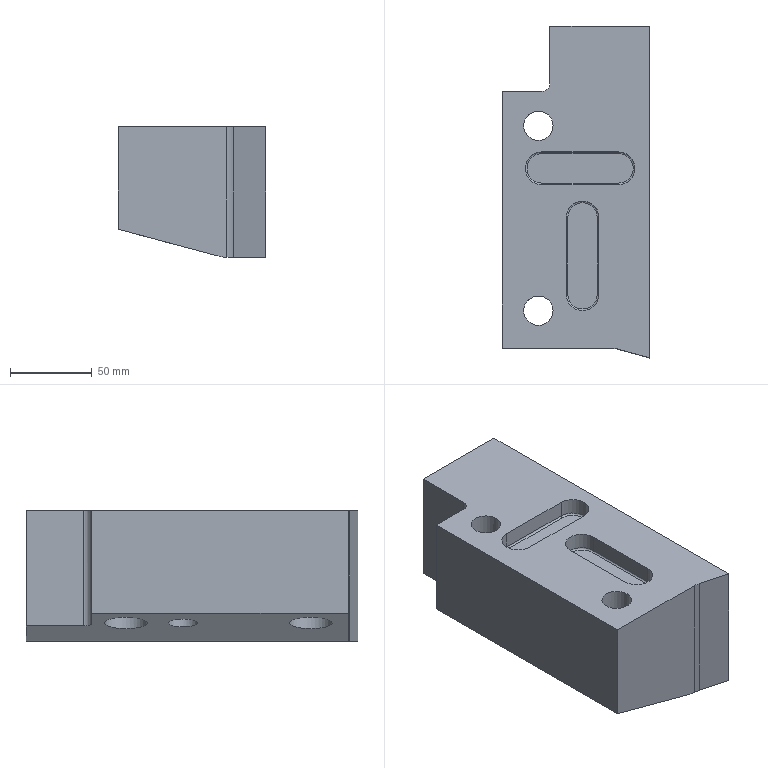Part | STEP file | lll_id3502_x_t | 1 solid | 41 faces | box 90 x 202.78 x 80 mm | volume 1153649 mm3 | plane 19 | cylinder 17 | torus 4 | cone 1 | commonest cylinder face diameters 2 x4 20 x4 18.009 x2 26.008 x2 10 x1 14.505 x1
STEP:
#1=CARTESIAN_POINT('',(1694.772,-17.,3.437));
#2=VERTEX_POINT('',#1);
#3=CARTESIAN_POINT('',(1663.,-17.,11.95));
#4=VERTEX_POINT('',#3);
#5=CARTESIAN_POINT('',(1668.26,-17.,10.541));
#6=DIRECTION('',(-0.9659,0.,0.2588));
#7=VECTOR('',#6,1.);
#8=LINE('',#5,#7);
#9=EDGE_CURVE('',#2,#4,#8,.T.);
#10=ORIENTED_EDGE('',*,*,#9,.T.);
#11=CARTESIAN_POINT('',(1663.,-17.,82.5));
#12=VERTEX_POINT('',#11);
#13=CARTESIAN_POINT('',(1663.,-17.,-18.));
#14=DIRECTION('',(0.,0.,1.));
#15=VECTOR('',#14,1.);
#16=LINE('',#13,#15);
#17=EDGE_CURVE('',#4,#12,#16,.T.);
#18=ORIENTED_EDGE('',*,*,#17,.T.);
#19=CARTESIAN_POINT('',(1724.,-17.,82.5));
#20=VERTEX_POINT('',#19);
#21=CARTESIAN_POINT('',(1644.,-17.,82.5));
#22=DIRECTION('',(-1.,0.,0.));
#23=VECTOR('',#22,1.);
#24=LINE('',#21,#23);
#25=EDGE_CURVE('',#20,#12,#24,.T.);
#26=ORIENTED_EDGE('',*,*,#25,.F.);
#27=CARTESIAN_POINT('',(1724.,-17.,2.5));
#28=VERTEX_POINT('',#27);
#29=CARTESIAN_POINT('',(1724.,-17.,-80.));
#30=DIRECTION('',(0.,0.,1.));
#31=VECTOR('',#30,1.);
#32=LINE('',#29,#31);
#33=EDGE_CURVE('',#28,#20,#32,.T.);
#34=ORIENTED_EDGE('',*,*,#33,.F.);
#35=CARTESIAN_POINT('',(1701.89,-17.,2.5));
#36=VERTEX_POINT('',#35);
#37=CARTESIAN_POINT('',(12283.883,-17.,2.5));
#38=DIRECTION('',(-1.,0.,0.));
#39=VECTOR('',#38,1.);
#40=LINE('',#37,#39);
#41=EDGE_CURVE('',#28,#36,#40,.T.);
#42=ORIENTED_EDGE('',*,*,#41,.T.);
#43=CARTESIAN_POINT('',(1701.89,-17.,30.));
#44=DIRECTION('',(0.,-1.,0.));
#45=DIRECTION('',(0.,0.,1.));
#46=AXIS2_PLACEMENT_3D('',#43,#44,#45);
#47=CIRCLE('',#46,27.5);
#48=EDGE_CURVE('',#2,#36,#47,.T.);
#49=ORIENTED_EDGE('',*,*,#48,.F.);
#50=EDGE_LOOP('',(#10,#18,#26,#34,#42,#49));
#51=FACE_OUTER_BOUND('',#50,.T.);
#52=CARTESIAN_POINT('',(1644.,-17.,-80.));
#53=DIRECTION('',(0.,1.,0.));
#54=DIRECTION('',(0.,0.,1.));
#55=AXIS2_PLACEMENT_3D('',#52,#53,#54);
#56=PLANE('',#55);
#57=ADVANCED_FACE('',(#51),#56,.T.);
#58=ORIENTED_EDGE('',*,*,#41,.F.);
#59=CARTESIAN_POINT('',(1724.,-219.78,2.5));
#60=VERTEX_POINT('',#59);
#61=CARTESIAN_POINT('',(1724.,13712.786,2.5));
#62=DIRECTION('',(0.,-1.,0.));
#63=VECTOR('',#62,1.);
#64=LINE('',#61,#63);
#65=EDGE_CURVE('',#28,#60,#64,.T.);
#66=ORIENTED_EDGE('',*,*,#65,.T.);
#67=CARTESIAN_POINT('',(1704.214,-214.417,2.5));
#68=VERTEX_POINT('',#67);
#69=CARTESIAN_POINT('',(8043.284,-1932.589,2.5));
#70=DIRECTION('',(-0.9652,0.2616,0.));
#71=VECTOR('',#70,1.);
#72=LINE('',#69,#71);
#73=EDGE_CURVE('',#60,#68,#72,.T.);
#74=ORIENTED_EDGE('',*,*,#73,.T.);
#75=CARTESIAN_POINT('',(1701.89,-213.974,2.5));
#76=VERTEX_POINT('',#75);
#77=CARTESIAN_POINT('',(1700.159,-229.377,2.5));
#78=DIRECTION('',(0.,0.,-1.));
#79=DIRECTION('',(0.,1.,0.));
#80=AXIS2_PLACEMENT_3D('',#77,#78,#79);
#81=CIRCLE('',#80,15.5);
#82=EDGE_CURVE('',#76,#68,#81,.T.);
#83=ORIENTED_EDGE('',*,*,#82,.F.);
#84=CARTESIAN_POINT('',(1701.89,22.5,2.5));
#85=DIRECTION('',(0.,-1.,0.));
#86=VECTOR('',#85,1.);
#87=LINE('',#84,#86);
#88=EDGE_CURVE('',#36,#76,#87,.T.);
#89=ORIENTED_EDGE('',*,*,#88,.F.);
#90=EDGE_LOOP('',(#58,#66,#74,#83,#89));
#91=FACE_OUTER_BOUND('',#90,.T.);
#92=CARTESIAN_POINT('',(12283.883,13712.786,2.5));
#93=DIRECTION('',(0.,0.,-1.));
#94=DIRECTION('',(1.,0.,0.));
#95=AXIS2_PLACEMENT_3D('',#92,#93,#94);
#96=PLANE('',#95);
#97=ADVANCED_FACE('',(#91),#96,.T.);
#98=ORIENTED_EDGE('',*,*,#73,.F.);
#99=CARTESIAN_POINT('',(1724.,-219.78,82.5));
#100=VERTEX_POINT('',#99);
#101=CARTESIAN_POINT('',(1724.,-219.78,-7.5));
#102=DIRECTION('',(0.,0.,1.));
#103=VECTOR('',#102,1.);
#104=LINE('',#101,#103);
#105=EDGE_CURVE('',#60,#100,#104,.T.);
#106=ORIENTED_EDGE('',*,*,#105,.T.);
#107=CARTESIAN_POINT('',(1704.214,-214.417,82.5));
#108=VERTEX_POINT('',#107);
#109=CARTESIAN_POINT('',(1799.799,-240.325,82.5));
#110=DIRECTION('',(0.9652,-0.2616,0.));
#111=VECTOR('',#110,1.);
#112=LINE('',#109,#111);
#113=EDGE_CURVE('',#108,#100,#112,.T.);
#114=ORIENTED_EDGE('',*,*,#113,.F.);
#115=CARTESIAN_POINT('',(1704.214,-214.417,-7.5));
#116=DIRECTION('',(0.,0.,1.));
#117=VECTOR('',#116,1.);
#118=LINE('',#115,#117);
#119=EDGE_CURVE('',#68,#108,#118,.T.);
#120=ORIENTED_EDGE('',*,*,#119,.F.);
#121=EDGE_LOOP('',(#98,#106,#114,#120));
#122=FACE_OUTER_BOUND('',#121,.T.);
#123=CARTESIAN_POINT('',(1799.799,-240.325,-7.5));
#124=DIRECTION('',(-0.2616,-0.9652,0.));
#125=DIRECTION('',(-0.9652,0.2616,0.));
#126=AXIS2_PLACEMENT_3D('',#123,#124,#125);
#127=PLANE('',#126);
#128=ADVANCED_FACE('',(#122),#127,.T.);
#129=CARTESIAN_POINT('',(1673.,-181.,82.5));
#130=VERTEX_POINT('',#129);
#131=CARTESIAN_POINT('',(1673.,-134.,82.5));
#132=VERTEX_POINT('',#131);
#133=CARTESIAN_POINT('',(1673.,0.,82.5));
#134=DIRECTION('',(0.,1.,0.));
#135=VECTOR('',#134,1.);
#136=LINE('',#133,#135);
#137=EDGE_CURVE('',#130,#132,#136,.T.);
#138=ORIENTED_EDGE('',*,*,#137,.T.);
#139=CARTESIAN_POINT('',(1693.,-134.,82.5));
#140=VERTEX_POINT('',#139);
#141=CARTESIAN_POINT('',(1683.,-134.,82.5));
#142=DIRECTION('',(0.,0.,-1.));
#143=DIRECTION('',(-1.,0.,0.));
#144=AXIS2_PLACEMENT_3D('',#141,#142,#143);
#145=CIRCLE('',#144,10.);
#146=EDGE_CURVE('',#132,#140,#145,.T.);
#147=ORIENTED_EDGE('',*,*,#146,.T.);
#148=CARTESIAN_POINT('',(1693.,-181.,82.5));
#149=VERTEX_POINT('',#148);
#150=CARTESIAN_POINT('',(1693.,0.,82.5));
#151=DIRECTION('',(0.,-1.,0.));
#152=VECTOR('',#151,1.);
#153=LINE('',#150,#152);
#154=EDGE_CURVE('',#140,#149,#153,.T.);
#155=ORIENTED_EDGE('',*,*,#154,.T.);
#156=CARTESIAN_POINT('',(1683.,-181.,82.5));
#157=DIRECTION('',(0.,0.,-1.));
#158=DIRECTION('',(-1.,0.,0.));
#159=AXIS2_PLACEMENT_3D('',#156,#157,#158);
#160=CIRCLE('',#159,10.);
#161=EDGE_CURVE('',#149,#130,#160,.T.);
#162=ORIENTED_EDGE('',*,*,#161,.T.);
#163=EDGE_LOOP('',(#138,#147,#155,#162));
#164=FACE_BOUND('',#163,.T.);
#165=CARTESIAN_POINT('',(1705.,-114.,82.5));
#166=VERTEX_POINT('',#165);
#167=CARTESIAN_POINT('',(1658.,-114.,82.5));
#168=VERTEX_POINT('',#167);
#169=CARTESIAN_POINT('',(2347.435,-114.,82.5));
#170=DIRECTION('',(-1.,0.,0.));
#171=VECTOR('',#170,1.);
#172=LINE('',#169,#171);
#173=EDGE_CURVE('',#166,#168,#172,.T.);
#174=ORIENTED_EDGE('',*,*,#173,.T.);
#175=CARTESIAN_POINT('',(1658.,-94.,82.5));
#176=VERTEX_POINT('',#175);
#177=CARTESIAN_POINT('',(1658.,-104.,82.5));
#178=DIRECTION('',(0.,0.,-1.));
#179=DIRECTION('',(-1.,0.,0.));
#180=AXIS2_PLACEMENT_3D('',#177,#178,#179);
#181=CIRCLE('',#180,10.);
#182=EDGE_CURVE('',#168,#176,#181,.T.);
#183=ORIENTED_EDGE('',*,*,#182,.T.);
#184=CARTESIAN_POINT('',(1705.,-94.,82.5));
#185=VERTEX_POINT('',#184);
#186=CARTESIAN_POINT('',(2347.435,-94.,82.5));
#187=DIRECTION('',(1.,0.,0.));
#188=VECTOR('',#187,1.);
#189=LINE('',#186,#188);
#190=EDGE_CURVE('',#176,#185,#189,.T.);
#191=ORIENTED_EDGE('',*,*,#190,.T.);
#192=CARTESIAN_POINT('',(1705.,-104.,82.5));
#193=DIRECTION('',(0.,0.,-1.));
#194=DIRECTION('',(-1.,0.,0.));
#195=AXIS2_PLACEMENT_3D('',#192,#193,#194);
#196=CIRCLE('',#195,10.);
#197=EDGE_CURVE('',#185,#166,#196,.T.);
#198=ORIENTED_EDGE('',*,*,#197,.T.);
#199=EDGE_LOOP('',(#174,#183,#191,#198));
#200=FACE_BOUND('',#199,.T.);
#201=ORIENTED_EDGE('',*,*,#25,.T.);
#202=CARTESIAN_POINT('',(1663.,-52.,82.5));
#203=VERTEX_POINT('',#202);
#204=CARTESIAN_POINT('',(1663.,0.,82.5));
#205=DIRECTION('',(0.,-1.,0.));
#206=VECTOR('',#205,1.);
#207=LINE('',#204,#206);
#208=EDGE_CURVE('',#12,#203,#207,.T.);
#209=ORIENTED_EDGE('',*,*,#208,.T.);
#210=CARTESIAN_POINT('',(1658.,-57.,82.5));
#211=VERTEX_POINT('',#210);
#212=CARTESIAN_POINT('',(1658.,-52.,82.5));
#213=DIRECTION('',(0.,0.,-1.));
#214=DIRECTION('',(-1.,0.,0.));
#215=AXIS2_PLACEMENT_3D('',#212,#213,#214);
#216=CIRCLE('',#215,5.);
#217=EDGE_CURVE('',#203,#211,#216,.T.);
#218=ORIENTED_EDGE('',*,*,#217,.T.);
#219=CARTESIAN_POINT('',(1634.,-57.,82.5));
#220=VERTEX_POINT('',#219);
#221=CARTESIAN_POINT('',(2347.435,-57.,82.5));
#222=DIRECTION('',(-1.,0.,0.));
#223=VECTOR('',#222,1.);
#224=LINE('',#221,#223);
#225=EDGE_CURVE('',#211,#220,#224,.T.);
#226=ORIENTED_EDGE('',*,*,#225,.T.);
#227=CARTESIAN_POINT('',(1634.,-213.877,82.5));
#228=VERTEX_POINT('',#227);
#229=CARTESIAN_POINT('',(1634.,0.,82.5));
#230=DIRECTION('',(0.,1.,0.));
#231=VECTOR('',#230,1.);
#232=LINE('',#229,#231);
#233=EDGE_CURVE('',#228,#220,#232,.T.);
#234=ORIENTED_EDGE('',*,*,#233,.F.);
#235=CARTESIAN_POINT('',(1700.159,-213.877,82.5));
#236=VERTEX_POINT('',#235);
#237=CARTESIAN_POINT('',(2347.435,-213.877,82.5));
#238=DIRECTION('',(-1.,0.,0.));
#239=VECTOR('',#238,1.);
#240=LINE('',#237,#239);
#241=EDGE_CURVE('',#236,#228,#240,.T.);
#242=ORIENTED_EDGE('',*,*,#241,.F.);
#243=CARTESIAN_POINT('',(1700.159,-229.377,82.5));
#244=DIRECTION('',(0.,0.,-1.));
#245=DIRECTION('',(-1.,0.,0.));
#246=AXIS2_PLACEMENT_3D('',#243,#244,#245);
#247=CIRCLE('',#246,15.5);
#248=EDGE_CURVE('',#236,#108,#247,.T.);
#249=ORIENTED_EDGE('',*,*,#248,.T.);
#250=ORIENTED_EDGE('',*,*,#113,.T.);
#251=CARTESIAN_POINT('',(1724.,0.,82.5));
#252=DIRECTION('',(0.,-1.,0.));
#253=VECTOR('',#252,1.);
#254=LINE('',#251,#253);
#255=EDGE_CURVE('',#20,#100,#254,.T.);
#256=ORIENTED_EDGE('',*,*,#255,.F.);
#257=EDGE_LOOP('',(#201,#209,#218,#226,#234,#242,#249,#250,#256));
#258=FACE_BOUND('',#257,.T.);
#259=CARTESIAN_POINT('',(1665.005,-191.,82.5));
#260=VERTEX_POINT('',#259);
#261=CARTESIAN_POINT('',(1656.,-191.,82.5));
#262=DIRECTION('',(0.,0.,-1.));
#263=DIRECTION('',(1.,0.,0.));
#264=AXIS2_PLACEMENT_3D('',#261,#262,#263);
#265=CIRCLE('',#264,9.005);
#266=EDGE_CURVE('',#260,#260,#265,.T.);
#267=ORIENTED_EDGE('',*,*,#266,.T.);
#268=EDGE_LOOP('',(#267));
#269=FACE_BOUND('',#268,.T.);
#270=CARTESIAN_POINT('',(1665.005,-78.,82.5));
#271=VERTEX_POINT('',#270);
#272=CARTESIAN_POINT('',(1656.,-78.,82.5));
#273=DIRECTION('',(0.,0.,-1.));
#274=DIRECTION('',(1.,0.,0.));
#275=AXIS2_PLACEMENT_3D('',#272,#273,#274);
#276=CIRCLE('',#275,9.005);
#277=EDGE_CURVE('',#271,#271,#276,.T.);
#278=ORIENTED_EDGE('',*,*,#277,.T.);
#279=EDGE_LOOP('',(#278));
#280=FACE_BOUND('',#279,.T.);
#281=CARTESIAN_POINT('',(2347.435,0.,82.5));
#282=DIRECTION('',(0.,0.,-1.));
#283=DIRECTION('',(1.,0.,0.));
#284=AXIS2_PLACEMENT_3D('',#281,#282,#283);
#285=PLANE('',#284);
#286=ADVANCED_FACE('',(#164,#200,#258,#269,#280),#285,.F.);
#287=CARTESIAN_POINT('',(1647.,-113.,16.238));
#288=VERTEX_POINT('',#287);
#289=CARTESIAN_POINT('',(1656.,-113.,13.826));
#290=DIRECTION('',(-0.2588,0.,-0.9659));
#291=DIRECTION('',(-0.9659,0.,0.2588));
#292=AXIS2_PLACEMENT_3D('',#289,#290,#291);
#293=ELLIPSE('',#292,9.317,9.);
#294=EDGE_CURVE('',#288,#288,#293,.T.);
#295=ORIENTED_EDGE('',*,*,#294,.F.);
#296=EDGE_LOOP('',(#295));
#297=FACE_BOUND('',#296,.T.);
#298=CARTESIAN_POINT('',(1663.,-52.,11.95));
#299=VERTEX_POINT('',#298);
#300=CARTESIAN_POINT('',(1663.,22.5,11.95));
#301=DIRECTION('',(0.,-1.,0.));
#302=VECTOR('',#301,1.);
#303=LINE('',#300,#302);
#304=EDGE_CURVE('',#4,#299,#303,.T.);
#305=ORIENTED_EDGE('',*,*,#304,.F.);
#306=ORIENTED_EDGE('',*,*,#9,.F.);
#307=CARTESIAN_POINT('',(1694.772,-213.877,3.437));
#308=VERTEX_POINT('',#307);
#309=CARTESIAN_POINT('',(1694.772,22.5,3.437));
#310=DIRECTION('',(0.,-1.,0.));
#311=VECTOR('',#310,1.);
#312=LINE('',#309,#311);
#313=EDGE_CURVE('',#2,#308,#312,.T.);
#314=ORIENTED_EDGE('',*,*,#313,.T.);
#315=CARTESIAN_POINT('',(1634.,-213.877,19.721));
#316=VERTEX_POINT('',#315);
#317=CARTESIAN_POINT('',(1698.662,-213.877,2.395));
#318=DIRECTION('',(0.9659,0.,-0.2588));
#319=VECTOR('',#318,1.);
#320=LINE('',#317,#319);
#321=EDGE_CURVE('',#316,#308,#320,.T.);
#322=ORIENTED_EDGE('',*,*,#321,.F.);
#323=CARTESIAN_POINT('',(1634.,-57.,19.721));
#324=VERTEX_POINT('',#323);
#325=CARTESIAN_POINT('',(1634.,22.5,19.721));
#326=DIRECTION('',(0.,1.,0.));
#327=VECTOR('',#326,1.);
#328=LINE('',#325,#327);
#329=EDGE_CURVE('',#316,#324,#328,.T.);
#330=ORIENTED_EDGE('',*,*,#329,.T.);
#331=CARTESIAN_POINT('',(1658.,-57.,13.29));
#332=VERTEX_POINT('',#331);
#333=CARTESIAN_POINT('',(1774.42,-57.,-17.905));
#334=DIRECTION('',(-0.9659,0.,0.2588));
#335=VECTOR('',#334,1.);
#336=LINE('',#333,#335);
#337=EDGE_CURVE('',#332,#324,#336,.T.);
#338=ORIENTED_EDGE('',*,*,#337,.F.);
#339=CARTESIAN_POINT('',(1658.,-52.,13.29));
#340=DIRECTION('',(0.2588,0.,0.9659));
#341=DIRECTION('',(-0.9659,0.,0.2588));
#342=AXIS2_PLACEMENT_3D('',#339,#340,#341);
#343=ELLIPSE('',#342,5.176,5.);
#344=EDGE_CURVE('',#332,#299,#343,.T.);
#345=ORIENTED_EDGE('',*,*,#344,.T.);
#346=EDGE_LOOP('',(#305,#306,#314,#322,#330,#338,#345));
#347=FACE_BOUND('',#346,.T.);
#348=CARTESIAN_POINT('',(1642.996,-191.,17.31));
#349=VERTEX_POINT('',#348);
#350=CARTESIAN_POINT('',(1656.,-191.,13.826));
#351=DIRECTION('',(-0.2588,0.,-0.9659));
#352=DIRECTION('',(-0.9659,0.,0.2588));
#353=AXIS2_PLACEMENT_3D('',#350,#351,#352);
#354=ELLIPSE('',#353,13.463,13.004);
#355=EDGE_CURVE('',#349,#349,#354,.T.);
#356=ORIENTED_EDGE('',*,*,#355,.F.);
#357=EDGE_LOOP('',(#356));
#358=FACE_BOUND('',#357,.T.);
#359=CARTESIAN_POINT('',(1642.996,-78.,17.31));
#360=VERTEX_POINT('',#359);
#361=CARTESIAN_POINT('',(1656.,-78.,13.826));
#362=DIRECTION('',(-0.2588,0.,-0.9659));
#363=DIRECTION('',(-0.9659,0.,0.2588));
#364=AXIS2_PLACEMENT_3D('',#361,#362,#363);
#365=ELLIPSE('',#364,13.463,13.004);
#366=EDGE_CURVE('',#360,#360,#365,.T.);
#367=ORIENTED_EDGE('',*,*,#366,.F.);
#368=EDGE_LOOP('',(#367));
#369=FACE_BOUND('',#368,.T.);
#370=CARTESIAN_POINT('',(1774.42,22.5,-17.905));
#371=DIRECTION('',(-0.2588,0.,-0.9659));
#372=DIRECTION('',(0.9659,0.,-0.2588));
#373=AXIS2_PLACEMENT_3D('',#370,#371,#372);
#374=PLANE('',#373);
#375=ADVANCED_FACE('',(#297,#347,#358,#369),#374,.T.);
#376=CARTESIAN_POINT('',(1700.159,-213.877,2.555));
#377=VERTEX_POINT('',#376);
#378=CARTESIAN_POINT('',(1700.159,-213.877,2.555));
#379=CARTESIAN_POINT('',(1700.736,-213.877,2.518));
#380=CARTESIAN_POINT('',(1701.315,-213.909,2.5));
#381=CARTESIAN_POINT('',(1701.89,-213.974,2.5));
#382=B_SPLINE_CURVE_WITH_KNOTS('',3,(#378,#379,#380,#381),.UNSPECIFIED.,.F.,.F.,(4,4),(0.,1.),.UNSPECIFIED.);
#383=EDGE_CURVE('',#377,#76,#382,.T.);
#384=ORIENTED_EDGE('',*,*,#383,.F.);
#385=CARTESIAN_POINT('',(1701.89,-213.877,30.));
#386=DIRECTION('',(0.,-1.,0.));
#387=DIRECTION('',(1.,0.,0.));
#388=AXIS2_PLACEMENT_3D('',#385,#386,#387);
#389=CIRCLE('',#388,27.5);
#390=EDGE_CURVE('',#308,#377,#389,.T.);
#391=ORIENTED_EDGE('',*,*,#390,.F.);
#392=ORIENTED_EDGE('',*,*,#313,.F.);
#393=ORIENTED_EDGE('',*,*,#48,.T.);
#394=ORIENTED_EDGE('',*,*,#88,.T.);
#395=EDGE_LOOP('',(#384,#391,#392,#393,#394));
#396=FACE_OUTER_BOUND('',#395,.T.);
#397=CARTESIAN_POINT('',(1701.89,22.5,30.));
#398=DIRECTION('',(0.,-1.,0.));
#399=DIRECTION('',(-1.,0.,0.));
#400=AXIS2_PLACEMENT_3D('',#397,#398,#399);
#401=CYLINDRICAL_SURFACE('',#400,27.5);
#402=ADVANCED_FACE('',(#396),#401,.T.);
#403=CARTESIAN_POINT('',(1634.,-57.,-80.));
#404=DIRECTION('',(0.,0.,1.));
#405=VECTOR('',#404,1.);
#406=LINE('',#403,#405);
#407=EDGE_CURVE('',#324,#220,#406,.T.);
#408=ORIENTED_EDGE('',*,*,#407,.F.);
#409=ORIENTED_EDGE('',*,*,#329,.F.);
#410=CARTESIAN_POINT('',(1634.,-213.877,-80.));
#411=DIRECTION('',(0.,0.,1.));
#412=VECTOR('',#411,1.);
#413=LINE('',#410,#412);
#414=EDGE_CURVE('',#316,#228,#413,.T.);
#415=ORIENTED_EDGE('',*,*,#414,.T.);
#416=ORIENTED_EDGE('',*,*,#233,.T.);
#417=EDGE_LOOP('',(#408,#409,#415,#416));
#418=FACE_OUTER_BOUND('',#417,.T.);
#419=CARTESIAN_POINT('',(1634.,-320.,-80.));
#420=DIRECTION('',(-1.,0.,0.));
#421=DIRECTION('',(0.,0.,-1.));
#422=AXIS2_PLACEMENT_3D('',#419,#420,#421);
#423=PLANE('',#422);
#424=ADVANCED_FACE('',(#418),#423,.T.);
#425=ORIENTED_EDGE('',*,*,#119,.T.);
#426=ORIENTED_EDGE('',*,*,#248,.F.);
#427=CARTESIAN_POINT('',(1700.159,-213.877,-7.5));
#428=DIRECTION('',(0.,0.,-1.));
#429=VECTOR('',#428,1.);
#430=LINE('',#427,#429);
#431=EDGE_CURVE('',#236,#377,#430,.T.);
#432=ORIENTED_EDGE('',*,*,#431,.T.);
#433=ORIENTED_EDGE('',*,*,#383,.T.);
#434=ORIENTED_EDGE('',*,*,#82,.T.);
#435=EDGE_LOOP('',(#425,#426,#432,#433,#434));
#436=FACE_OUTER_BOUND('',#435,.T.);
#437=CARTESIAN_POINT('',(1700.159,-229.377,-7.5));
#438=DIRECTION('',(0.,0.,-1.));
#439=DIRECTION('',(1.,0.,0.));
#440=AXIS2_PLACEMENT_3D('',#437,#438,#439);
#441=CYLINDRICAL_SURFACE('',#440,15.5);
#442=ADVANCED_FACE('',(#436),#441,.F.);
#443=ORIENTED_EDGE('',*,*,#241,.T.);
#444=ORIENTED_EDGE('',*,*,#414,.F.);
#445=ORIENTED_EDGE('',*,*,#321,.T.);
#446=ORIENTED_EDGE('',*,*,#390,.T.);
#447=ORIENTED_EDGE('',*,*,#431,.F.);
#448=EDGE_LOOP('',(#443,#444,#445,#446,#447));
#449=FACE_OUTER_BOUND('',#448,.T.);
#450=CARTESIAN_POINT('',(1696.172,-213.877,-6.899));
#451=DIRECTION('',(0.,-1.,0.));
#452=DIRECTION('',(-1.,0.,0.));
#453=AXIS2_PLACEMENT_3D('',#450,#451,#452);
#454=PLANE('',#453);
#455=ADVANCED_FACE('',(#449),#454,.T.);
#456=ORIENTED_EDGE('',*,*,#33,.T.);
#457=ORIENTED_EDGE('',*,*,#255,.T.);
#458=ORIENTED_EDGE('',*,*,#105,.F.);
#459=ORIENTED_EDGE('',*,*,#65,.F.);
#460=EDGE_LOOP('',(#456,#457,#458,#459));
#461=FACE_OUTER_BOUND('',#460,.T.);
#462=CARTESIAN_POINT('',(1724.,124.058,42.5));
#463=DIRECTION('',(1.,0.,0.));
#464=DIRECTION('',(0.,0.,1.));
#465=AXIS2_PLACEMENT_3D('',#462,#463,#464);
#466=PLANE('',#465);
#467=ADVANCED_FACE('',(#461),#466,.T.);
#468=CARTESIAN_POINT('',(1656.,-87.004,42.5));
#469=VERTEX_POINT('',#468);
#470=CARTESIAN_POINT('',(1656.,-78.,42.5));
#471=DIRECTION('',(0.,0.,1.));
#472=DIRECTION('',(0.,-1.,0.));
#473=AXIS2_PLACEMENT_3D('',#470,#471,#472);
#474=CIRCLE('',#473,9.005);
#475=EDGE_CURVE('',#469,#469,#474,.T.);
#476=ORIENTED_EDGE('',*,*,#475,.F.);
#477=EDGE_LOOP('',(#476));
#478=FACE_BOUND('',#477,.T.);
#479=ORIENTED_EDGE('',*,*,#277,.F.);
#480=EDGE_LOOP('',(#479));
#481=FACE_BOUND('',#480,.T.);
#482=CARTESIAN_POINT('',(1656.,-78.,2.5));
#483=DIRECTION('',(0.,0.,1.));
#484=DIRECTION('',(1.,0.,0.));
#485=AXIS2_PLACEMENT_3D('',#482,#483,#484);
#486=CYLINDRICAL_SURFACE('',#485,9.005);
#487=ADVANCED_FACE('',(#478,#481),#486,.F.);
#488=ORIENTED_EDGE('',*,*,#475,.T.);
#489=EDGE_LOOP('',(#488));
#490=FACE_BOUND('',#489,.T.);
#491=CARTESIAN_POINT('',(1669.004,-78.,42.5));
#492=VERTEX_POINT('',#491);
#493=CARTESIAN_POINT('',(1656.,-78.,42.5));
#494=DIRECTION('',(0.,0.,1.));
#495=DIRECTION('',(1.,0.,0.));
#496=AXIS2_PLACEMENT_3D('',#493,#494,#495);
#497=CIRCLE('',#496,13.004);
#498=EDGE_CURVE('',#492,#492,#497,.T.);
#499=ORIENTED_EDGE('',*,*,#498,.F.);
#500=EDGE_LOOP('',(#499));
#501=FACE_BOUND('',#500,.T.);
#502=CARTESIAN_POINT('',(1656.,-78.,42.5));
#503=DIRECTION('',(0.,0.,1.));
#504=DIRECTION('',(0.,-1.,0.));
#505=AXIS2_PLACEMENT_3D('',#502,#503,#504);
#506=PLANE('',#505);
#507=ADVANCED_FACE('',(#490,#501),#506,.F.);
#508=ORIENTED_EDGE('',*,*,#366,.T.);
#509=EDGE_LOOP('',(#508));
#510=FACE_BOUND('',#509,.T.);
#511=ORIENTED_EDGE('',*,*,#498,.T.);
#512=EDGE_LOOP('',(#511));
#513=FACE_BOUND('',#512,.T.);
#514=CARTESIAN_POINT('',(1656.,-78.,2.5));
#515=DIRECTION('',(0.,0.,1.));
#516=DIRECTION('',(1.,0.,0.));
#517=AXIS2_PLACEMENT_3D('',#514,#515,#516);
#518=CYLINDRICAL_SURFACE('',#517,13.004);
#519=ADVANCED_FACE('',(#510,#513),#518,.F.);
#520=CARTESIAN_POINT('',(1656.,-200.004,42.5));
#521=VERTEX_POINT('',#520);
#522=CARTESIAN_POINT('',(1656.,-191.,42.5));
#523=DIRECTION('',(0.,0.,1.));
#524=DIRECTION('',(0.,-1.,0.));
#525=AXIS2_PLACEMENT_3D('',#522,#523,#524);
#526=CIRCLE('',#525,9.005);
#527=EDGE_CURVE('',#521,#521,#526,.T.);
#528=ORIENTED_EDGE('',*,*,#527,.F.);
#529=EDGE_LOOP('',(#528));
#530=FACE_BOUND('',#529,.T.);
#531=ORIENTED_EDGE('',*,*,#266,.F.);
#532=EDGE_LOOP('',(#531));
#533=FACE_BOUND('',#532,.T.);
#534=CARTESIAN_POINT('',(1656.,-191.,2.5));
#535=DIRECTION('',(0.,0.,1.));
#536=DIRECTION('',(1.,0.,0.));
#537=AXIS2_PLACEMENT_3D('',#534,#535,#536);
#538=CYLINDRICAL_SURFACE('',#537,9.005);
#539=ADVANCED_FACE('',(#530,#533),#538,.F.);
#540=ORIENTED_EDGE('',*,*,#527,.T.);
#541=EDGE_LOOP('',(#540));
#542=FACE_BOUND('',#541,.T.);
#543=CARTESIAN_POINT('',(1669.004,-191.,42.5));
#544=VERTEX_POINT('',#543);
#545=CARTESIAN_POINT('',(1656.,-191.,42.5));
#546=DIRECTION('',(0.,0.,1.));
#547=DIRECTION('',(1.,0.,0.));
#548=AXIS2_PLACEMENT_3D('',#545,#546,#547);
#549=CIRCLE('',#548,13.004);
#550=EDGE_CURVE('',#544,#544,#549,.T.);
#551=ORIENTED_EDGE('',*,*,#550,.F.);
#552=EDGE_LOOP('',(#551));
#553=FACE_BOUND('',#552,.T.);
#554=CARTESIAN_POINT('',(1656.,-191.,42.5));
#555=DIRECTION('',(0.,0.,1.));
#556=DIRECTION('',(0.,-1.,0.));
#557=AXIS2_PLACEMENT_3D('',#554,#555,#556);
#558=PLANE('',#557);
#559=ADVANCED_FACE('',(#542,#553),#558,.F.);
#560=ORIENTED_EDGE('',*,*,#355,.T.);
#561=EDGE_LOOP('',(#560));
#562=FACE_BOUND('',#561,.T.);
#563=ORIENTED_EDGE('',*,*,#550,.T.);
#564=EDGE_LOOP('',(#563));
#565=FACE_BOUND('',#564,.T.);
#566=CARTESIAN_POINT('',(1656.,-191.,2.5));
#567=DIRECTION('',(0.,0.,1.));
#568=DIRECTION('',(1.,0.,0.));
#569=AXIS2_PLACEMENT_3D('',#566,#567,#568);
#570=CYLINDRICAL_SURFACE('',#569,13.004);
#571=ADVANCED_FACE('',(#562,#565),#570,.F.);
#572=ORIENTED_EDGE('',*,*,#304,.T.);
#573=CARTESIAN_POINT('',(1663.,-52.,82.5));
#574=DIRECTION('',(0.,0.,1.));
#575=VECTOR('',#574,1.);
#576=LINE('',#573,#575);
#577=EDGE_CURVE('',#299,#203,#576,.T.);
#578=ORIENTED_EDGE('',*,*,#577,.T.);
#579=ORIENTED_EDGE('',*,*,#208,.F.);
#580=ORIENTED_EDGE('',*,*,#17,.F.);
#581=EDGE_LOOP('',(#572,#578,#579,#580));
#582=FACE_OUTER_BOUND('',#581,.T.);
#583=CARTESIAN_POINT('',(1663.,-40.5,-18.));
#584=DIRECTION('',(1.,0.,0.));
#585=DIRECTION('',(0.,0.,-1.));
#586=AXIS2_PLACEMENT_3D('',#583,#584,#585);
#587=PLANE('',#586);
#588=ADVANCED_FACE('',(#582),#587,.F.);
#589=ORIENTED_EDGE('',*,*,#225,.F.);
#590=CARTESIAN_POINT('',(1658.,-57.,10.152));
#591=DIRECTION('',(0.,0.,-1.));
#592=VECTOR('',#591,1.);
#593=LINE('',#590,#592);
#594=EDGE_CURVE('',#211,#332,#593,.T.);
#595=ORIENTED_EDGE('',*,*,#594,.T.);
#596=ORIENTED_EDGE('',*,*,#337,.T.);
#597=ORIENTED_EDGE('',*,*,#407,.T.);
#598=EDGE_LOOP('',(#589,#595,#596,#597));
#599=FACE_OUTER_BOUND('',#598,.T.);
#600=CARTESIAN_POINT('',(1625.,-57.,-18.));
#601=DIRECTION('',(0.,-1.,0.));
#602=DIRECTION('',(0.,0.,-1.));
#603=AXIS2_PLACEMENT_3D('',#600,#601,#602);
#604=PLANE('',#603);
#605=ADVANCED_FACE('',(#599),#604,.F.);
#606=ORIENTED_EDGE('',*,*,#217,.F.);
#607=ORIENTED_EDGE('',*,*,#577,.F.);
#608=ORIENTED_EDGE('',*,*,#344,.F.);
#609=ORIENTED_EDGE('',*,*,#594,.F.);
#610=EDGE_LOOP('',(#606,#607,#608,#609));
#611=FACE_OUTER_BOUND('',#610,.T.);
#612=CARTESIAN_POINT('',(1658.,-52.,-18.));
#613=DIRECTION('',(0.,0.,1.));
#614=DIRECTION('',(1.,0.,0.));
#615=AXIS2_PLACEMENT_3D('',#612,#613,#614);
#616=CYLINDRICAL_SURFACE('',#615,5.);
#617=ADVANCED_FACE('',(#611),#616,.F.);
#618=CARTESIAN_POINT('',(1705.,-114.,72.5));
#619=VERTEX_POINT('',#618);
#620=CARTESIAN_POINT('',(1705.,-114.,92.5));
#621=DIRECTION('',(0.,0.,-1.));
#622=VECTOR('',#621,1.);
#623=LINE('',#620,#622);
#624=EDGE_CURVE('',#166,#619,#623,.T.);
#625=ORIENTED_EDGE('',*,*,#624,.T.);
#626=CARTESIAN_POINT('',(1658.,-114.,72.5));
#627=VERTEX_POINT('',#626);
#628=CARTESIAN_POINT('',(1658.,-114.,72.5));
#629=DIRECTION('',(-1.,0.,0.));
#630=VECTOR('',#629,1.);
#631=LINE('',#628,#630);
#632=EDGE_CURVE('',#619,#627,#631,.T.);
#633=ORIENTED_EDGE('',*,*,#632,.T.);
#634=CARTESIAN_POINT('',(1658.,-114.,92.5));
#635=DIRECTION('',(0.,0.,1.));
#636=VECTOR('',#635,1.);
#637=LINE('',#634,#636);
#638=EDGE_CURVE('',#627,#168,#637,.T.);
#639=ORIENTED_EDGE('',*,*,#638,.T.);
#640=ORIENTED_EDGE('',*,*,#173,.F.);
#641=EDGE_LOOP('',(#625,#633,#639,#640));
#642=FACE_OUTER_BOUND('',#641,.T.);
#643=CARTESIAN_POINT('',(1681.5,-114.,92.5));
#644=DIRECTION('',(0.,-1.,0.));
#645=DIRECTION('',(0.,0.,1.));
#646=AXIS2_PLACEMENT_3D('',#643,#644,#645);
#647=PLANE('',#646);
#648=ADVANCED_FACE('',(#642),#647,.F.);
#649=CARTESIAN_POINT('',(1658.,-94.,72.5));
#650=VERTEX_POINT('',#649);
#651=CARTESIAN_POINT('',(1658.,-94.,92.5));
#652=DIRECTION('',(0.,0.,-1.));
#653=VECTOR('',#652,1.);
#654=LINE('',#651,#653);
#655=EDGE_CURVE('',#176,#650,#654,.T.);
#656=ORIENTED_EDGE('',*,*,#655,.T.);
#657=CARTESIAN_POINT('',(1705.,-94.,72.5));
#658=VERTEX_POINT('',#657);
#659=CARTESIAN_POINT('',(1705.,-94.,72.5));
#660=DIRECTION('',(1.,0.,0.));
#661=VECTOR('',#660,1.);
#662=LINE('',#659,#661);
#663=EDGE_CURVE('',#650,#658,#662,.T.);
#664=ORIENTED_EDGE('',*,*,#663,.T.);
#665=CARTESIAN_POINT('',(1705.,-94.,92.5));
#666=DIRECTION('',(0.,0.,1.));
#667=VECTOR('',#666,1.);
#668=LINE('',#665,#667);
#669=EDGE_CURVE('',#658,#185,#668,.T.);
#670=ORIENTED_EDGE('',*,*,#669,.T.);
#671=ORIENTED_EDGE('',*,*,#190,.F.);
#672=EDGE_LOOP('',(#656,#664,#670,#671));
#673=FACE_OUTER_BOUND('',#672,.T.);
#674=CARTESIAN_POINT('',(1681.5,-94.,92.5));
#675=DIRECTION('',(0.,1.,0.));
#676=DIRECTION('',(0.,0.,-1.));
#677=AXIS2_PLACEMENT_3D('',#674,#675,#676);
#678=PLANE('',#677);
#679=ADVANCED_FACE('',(#673),#678,.F.);
#680=ORIENTED_EDGE('',*,*,#638,.F.);
#681=CARTESIAN_POINT('',(1658.,-104.,72.5));
#682=DIRECTION('',(0.,0.,-1.));
#683=DIRECTION('',(1.,0.,0.));
#684=AXIS2_PLACEMENT_3D('',#681,#682,#683);
#685=CIRCLE('',#684,10.);
#686=EDGE_CURVE('',#627,#650,#685,.T.);
#687=ORIENTED_EDGE('',*,*,#686,.T.);
#688=ORIENTED_EDGE('',*,*,#655,.F.);
#689=ORIENTED_EDGE('',*,*,#182,.F.);
#690=EDGE_LOOP('',(#680,#687,#688,#689));
#691=FACE_OUTER_BOUND('',#690,.T.);
#692=CARTESIAN_POINT('',(1658.,-104.,92.5));
#693=DIRECTION('',(0.,0.,-1.));
#694=DIRECTION('',(0.,-1.,0.));
#695=AXIS2_PLACEMENT_3D('',#692,#693,#694);
#696=CYLINDRICAL_SURFACE('',#695,10.);
#697=ADVANCED_FACE('',(#691),#696,.F.);
#698=ORIENTED_EDGE('',*,*,#669,.F.);
#699=CARTESIAN_POINT('',(1705.,-104.,72.5));
#700=DIRECTION('',(0.,0.,-1.));
#701=DIRECTION('',(1.,0.,0.));
#702=AXIS2_PLACEMENT_3D('',#699,#700,#701);
#703=CIRCLE('',#702,10.);
#704=EDGE_CURVE('',#658,#619,#703,.T.);
#705=ORIENTED_EDGE('',*,*,#704,.T.);
#706=ORIENTED_EDGE('',*,*,#624,.F.);
#707=ORIENTED_EDGE('',*,*,#197,.F.);
#708=EDGE_LOOP('',(#698,#705,#706,#707));
#709=FACE_OUTER_BOUND('',#708,.T.);
#710=CARTESIAN_POINT('',(1705.,-104.,92.5));
#711=DIRECTION('',(0.,0.,-1.));
#712=DIRECTION('',(0.,-1.,0.));
#713=AXIS2_PLACEMENT_3D('',#710,#711,#712);
#714=CYLINDRICAL_SURFACE('',#713,10.);
#715=ADVANCED_FACE('',(#709),#714,.F.);
#716=CARTESIAN_POINT('',(1658.,-113.,71.5));
#717=VERTEX_POINT('',#716);
#718=CARTESIAN_POINT('',(1705.,-113.,71.5));
#719=VERTEX_POINT('',#718);
#720=CARTESIAN_POINT('',(1705.,-113.,71.5));
#721=DIRECTION('',(1.,0.,0.));
#722=VECTOR('',#721,1.);
#723=LINE('',#720,#722);
#724=EDGE_CURVE('',#717,#719,#723,.T.);
#725=ORIENTED_EDGE('',*,*,#724,.T.);
#726=CARTESIAN_POINT('',(1705.,-95.,71.5));
#727=VERTEX_POINT('',#726);
#728=CARTESIAN_POINT('',(1705.,-104.,71.5));
#729=DIRECTION('',(0.,0.,1.));
#730=DIRECTION('',(1.,0.,0.));
#731=AXIS2_PLACEMENT_3D('',#728,#729,#730);
#732=CIRCLE('',#731,9.);
#733=EDGE_CURVE('',#719,#727,#732,.T.);
#734=ORIENTED_EDGE('',*,*,#733,.T.);
#735=CARTESIAN_POINT('',(1658.,-95.,71.5));
#736=VERTEX_POINT('',#735);
#737=CARTESIAN_POINT('',(1658.,-95.,71.5));
#738=DIRECTION('',(-1.,0.,0.));
#739=VECTOR('',#738,1.);
#740=LINE('',#737,#739);
#741=EDGE_CURVE('',#727,#736,#740,.T.);
#742=ORIENTED_EDGE('',*,*,#741,.T.);
#743=CARTESIAN_POINT('',(1658.,-104.,71.5));
#744=DIRECTION('',(0.,0.,1.));
#745=DIRECTION('',(1.,0.,0.));
#746=AXIS2_PLACEMENT_3D('',#743,#744,#745);
#747=CIRCLE('',#746,9.);
#748=EDGE_CURVE('',#736,#717,#747,.T.);
#749=ORIENTED_EDGE('',*,*,#748,.T.);
#750=EDGE_LOOP('',(#725,#734,#742,#749));
#751=FACE_OUTER_BOUND('',#750,.T.);
#752=CARTESIAN_POINT('',(1681.5,-104.,71.5));
#753=DIRECTION('',(0.,0.,1.));
#754=DIRECTION('',(0.,1.,0.));
#755=AXIS2_PLACEMENT_3D('',#752,#753,#754);
#756=PLANE('',#755);
#757=ADVANCED_FACE('',(#751),#756,.T.);
#758=CARTESIAN_POINT('',(1673.,-181.,72.5));
#759=VERTEX_POINT('',#758);
#760=CARTESIAN_POINT('',(1673.,-181.,92.5));
#761=DIRECTION('',(0.,0.,-1.));
#762=VECTOR('',#761,1.);
#763=LINE('',#760,#762);
#764=EDGE_CURVE('',#130,#759,#763,.T.);
#765=ORIENTED_EDGE('',*,*,#764,.T.);
#766=CARTESIAN_POINT('',(1673.,-134.,72.5));
#767=VERTEX_POINT('',#766);
#768=CARTESIAN_POINT('',(1673.,-134.,72.5));
#769=DIRECTION('',(0.,1.,0.));
#770=VECTOR('',#769,1.);
#771=LINE('',#768,#770);
#772=EDGE_CURVE('',#759,#767,#771,.T.);
#773=ORIENTED_EDGE('',*,*,#772,.T.);
#774=CARTESIAN_POINT('',(1673.,-134.,92.5));
#775=DIRECTION('',(0.,0.,1.));
#776=VECTOR('',#775,1.);
#777=LINE('',#774,#776);
#778=EDGE_CURVE('',#767,#132,#777,.T.);
#779=ORIENTED_EDGE('',*,*,#778,.T.);
#780=ORIENTED_EDGE('',*,*,#137,.F.);
#781=EDGE_LOOP('',(#765,#773,#779,#780));
#782=FACE_OUTER_BOUND('',#781,.T.);
#783=CARTESIAN_POINT('',(1673.,-157.5,92.5));
#784=DIRECTION('',(-1.,0.,0.));
#785=DIRECTION('',(0.,0.,1.));
#786=AXIS2_PLACEMENT_3D('',#783,#784,#785);
#787=PLANE('',#786);
#788=ADVANCED_FACE('',(#782),#787,.F.);
#789=CARTESIAN_POINT('',(1693.,-134.,72.5));
#790=VERTEX_POINT('',#789);
#791=CARTESIAN_POINT('',(1693.,-134.,92.5));
#792=DIRECTION('',(0.,0.,-1.));
#793=VECTOR('',#792,1.);
#794=LINE('',#791,#793);
#795=EDGE_CURVE('',#140,#790,#794,.T.);
#796=ORIENTED_EDGE('',*,*,#795,.T.);
#797=CARTESIAN_POINT('',(1693.,-181.,72.5));
#798=VERTEX_POINT('',#797);
#799=CARTESIAN_POINT('',(1693.,-181.,72.5));
#800=DIRECTION('',(0.,-1.,0.));
#801=VECTOR('',#800,1.);
#802=LINE('',#799,#801);
#803=EDGE_CURVE('',#790,#798,#802,.T.);
#804=ORIENTED_EDGE('',*,*,#803,.T.);
#805=CARTESIAN_POINT('',(1693.,-181.,92.5));
#806=DIRECTION('',(0.,0.,1.));
#807=VECTOR('',#806,1.);
#808=LINE('',#805,#807);
#809=EDGE_CURVE('',#798,#149,#808,.T.);
#810=ORIENTED_EDGE('',*,*,#809,.T.);
#811=ORIENTED_EDGE('',*,*,#154,.F.);
#812=EDGE_LOOP('',(#796,#804,#810,#811));
#813=FACE_OUTER_BOUND('',#812,.T.);
#814=CARTESIAN_POINT('',(1693.,-157.5,92.5));
#815=DIRECTION('',(1.,0.,0.));
#816=DIRECTION('',(0.,0.,-1.));
#817=AXIS2_PLACEMENT_3D('',#814,#815,#816);
#818=PLANE('',#817);
#819=ADVANCED_FACE('',(#813),#818,.F.);
#820=ORIENTED_EDGE('',*,*,#778,.F.);
#821=CARTESIAN_POINT('',(1683.,-134.,72.5));
#822=DIRECTION('',(0.,0.,-1.));
#823=DIRECTION('',(1.,0.,0.));
#824=AXIS2_PLACEMENT_3D('',#821,#822,#823);
#825=CIRCLE('',#824,10.);
#826=EDGE_CURVE('',#767,#790,#825,.T.);
#827=ORIENTED_EDGE('',*,*,#826,.T.);
#828=ORIENTED_EDGE('',*,*,#795,.F.);
#829=ORIENTED_EDGE('',*,*,#146,.F.);
#830=EDGE_LOOP('',(#820,#827,#828,#829));
#831=FACE_OUTER_BOUND('',#830,.T.);
#832=CARTESIAN_POINT('',(1683.,-134.,92.5));
#833=DIRECTION('',(0.,0.,-1.));
#834=DIRECTION('',(-1.,0.,0.));
#835=AXIS2_PLACEMENT_3D('',#832,#833,#834);
#836=CYLINDRICAL_SURFACE('',#835,10.);
#837=ADVANCED_FACE('',(#831),#836,.F.);
#838=ORIENTED_EDGE('',*,*,#809,.F.);
#839=CARTESIAN_POINT('',(1683.,-181.,72.5));
#840=DIRECTION('',(0.,0.,-1.));
#841=DIRECTION('',(1.,0.,0.));
#842=AXIS2_PLACEMENT_3D('',#839,#840,#841);
#843=CIRCLE('',#842,10.);
#844=EDGE_CURVE('',#798,#759,#843,.T.);
#845=ORIENTED_EDGE('',*,*,#844,.T.);
#846=ORIENTED_EDGE('',*,*,#764,.F.);
#847=ORIENTED_EDGE('',*,*,#161,.F.);
#848=EDGE_LOOP('',(#838,#845,#846,#847));
#849=FACE_OUTER_BOUND('',#848,.T.);
#850=CARTESIAN_POINT('',(1683.,-181.,92.5));
#851=DIRECTION('',(0.,0.,-1.));
#852=DIRECTION('',(-1.,0.,0.));
#853=AXIS2_PLACEMENT_3D('',#850,#851,#852);
#854=CYLINDRICAL_SURFACE('',#853,10.);
#855=ADVANCED_FACE('',(#849),#854,.F.);
#856=CARTESIAN_POINT('',(1674.,-134.,71.5));
#857=VERTEX_POINT('',#856);
#858=CARTESIAN_POINT('',(1674.,-181.,71.5));
#859=VERTEX_POINT('',#858);
#860=CARTESIAN_POINT('',(1674.,-181.,71.5));
#861=DIRECTION('',(0.,-1.,0.));
#862=VECTOR('',#861,1.);
#863=LINE('',#860,#862);
#864=EDGE_CURVE('',#857,#859,#863,.T.);
#865=ORIENTED_EDGE('',*,*,#864,.T.);
#866=CARTESIAN_POINT('',(1692.,-181.,71.5));
#867=VERTEX_POINT('',#866);
#868=CARTESIAN_POINT('',(1683.,-181.,71.5));
#869=DIRECTION('',(0.,0.,1.));
#870=DIRECTION('',(1.,0.,0.));
#871=AXIS2_PLACEMENT_3D('',#868,#869,#870);
#872=CIRCLE('',#871,9.);
#873=EDGE_CURVE('',#859,#867,#872,.T.);
#874=ORIENTED_EDGE('',*,*,#873,.T.);
#875=CARTESIAN_POINT('',(1692.,-134.,71.5));
#876=VERTEX_POINT('',#875);
#877=CARTESIAN_POINT('',(1692.,-134.,71.5));
#878=DIRECTION('',(0.,1.,0.));
#879=VECTOR('',#878,1.);
#880=LINE('',#877,#879);
#881=EDGE_CURVE('',#867,#876,#880,.T.);
#882=ORIENTED_EDGE('',*,*,#881,.T.);
#883=CARTESIAN_POINT('',(1683.,-134.,71.5));
#884=DIRECTION('',(0.,0.,1.));
#885=DIRECTION('',(1.,0.,0.));
#886=AXIS2_PLACEMENT_3D('',#883,#884,#885);
#887=CIRCLE('',#886,9.);
#888=EDGE_CURVE('',#876,#857,#887,.T.);
#889=ORIENTED_EDGE('',*,*,#888,.T.);
#890=EDGE_LOOP('',(#865,#874,#882,#889));
#891=FACE_OUTER_BOUND('',#890,.T.);
#892=CARTESIAN_POINT('',(1683.,-157.5,71.5));
#893=DIRECTION('',(0.,0.,1.));
#894=DIRECTION('',(1.,0.,0.));
#895=AXIS2_PLACEMENT_3D('',#892,#893,#894);
#896=PLANE('',#895);
#897=ADVANCED_FACE('',(#891),#896,.T.);
#898=CARTESIAN_POINT('',(1692.,-134.,72.5));
#899=DIRECTION('',(0.,1.,0.));
#900=DIRECTION('',(0.,0.,1.));
#901=AXIS2_PLACEMENT_3D('',#898,#899,#900);
#902=CIRCLE('',#901,1.);
#903=EDGE_CURVE('',#790,#876,#902,.T.);
#904=ORIENTED_EDGE('',*,*,#903,.F.);
#905=ORIENTED_EDGE('',*,*,#826,.F.);
#906=CARTESIAN_POINT('',(1674.,-134.,72.5));
#907=DIRECTION('',(0.,1.,0.));
#908=DIRECTION('',(0.,0.,1.));
#909=AXIS2_PLACEMENT_3D('',#906,#907,#908);
#910=CIRCLE('',#909,1.);
#911=EDGE_CURVE('',#857,#767,#910,.T.);
#912=ORIENTED_EDGE('',*,*,#911,.F.);
#913=ORIENTED_EDGE('',*,*,#888,.F.);
#914=EDGE_LOOP('',(#904,#905,#912,#913));
#915=FACE_OUTER_BOUND('',#914,.T.);
#916=CARTESIAN_POINT('',(1683.,-134.,72.5));
#917=DIRECTION('',(0.,0.,1.));
#918=DIRECTION('',(1.,0.,0.));
#919=AXIS2_PLACEMENT_3D('',#916,#917,#918);
#920=TOROIDAL_SURFACE('',#919,9.,1.);
#921=ADVANCED_FACE('',(#915),#920,.F.);
#922=ORIENTED_EDGE('',*,*,#911,.T.);
#923=ORIENTED_EDGE('',*,*,#772,.F.);
#924=CARTESIAN_POINT('',(1674.,-181.,72.5));
#925=DIRECTION('',(0.,1.,0.));
#926=DIRECTION('',(0.,0.,1.));
#927=AXIS2_PLACEMENT_3D('',#924,#925,#926);
#928=CIRCLE('',#927,1.);
#929=EDGE_CURVE('',#859,#759,#928,.T.);
#930=ORIENTED_EDGE('',*,*,#929,.F.);
#931=ORIENTED_EDGE('',*,*,#864,.F.);
#932=EDGE_LOOP('',(#922,#923,#930,#931));
#933=FACE_OUTER_BOUND('',#932,.T.);
#934=CARTESIAN_POINT('',(1674.,-157.5,72.5));
#935=DIRECTION('',(0.,1.,0.));
#936=DIRECTION('',(0.,0.,1.));
#937=AXIS2_PLACEMENT_3D('',#934,#935,#936);
#938=CYLINDRICAL_SURFACE('',#937,1.);
#939=ADVANCED_FACE('',(#933),#938,.F.);
#940=ORIENTED_EDGE('',*,*,#903,.T.);
#941=ORIENTED_EDGE('',*,*,#881,.F.);
#942=CARTESIAN_POINT('',(1692.,-181.,72.5));
#943=DIRECTION('',(0.,1.,0.));
#944=DIRECTION('',(0.,0.,1.));
#945=AXIS2_PLACEMENT_3D('',#942,#943,#944);
#946=CIRCLE('',#945,1.);
#947=EDGE_CURVE('',#798,#867,#946,.T.);
#948=ORIENTED_EDGE('',*,*,#947,.F.);
#949=ORIENTED_EDGE('',*,*,#803,.F.);
#950=EDGE_LOOP('',(#940,#941,#948,#949));
#951=FACE_OUTER_BOUND('',#950,.T.);
#952=CARTESIAN_POINT('',(1692.,-157.5,72.5));
#953=DIRECTION('',(0.,-1.,0.));
#954=DIRECTION('',(0.,0.,-1.));
#955=AXIS2_PLACEMENT_3D('',#952,#953,#954);
#956=CYLINDRICAL_SURFACE('',#955,1.);
#957=ADVANCED_FACE('',(#951),#956,.F.);
#958=ORIENTED_EDGE('',*,*,#929,.T.);
#959=ORIENTED_EDGE('',*,*,#844,.F.);
#960=ORIENTED_EDGE('',*,*,#947,.T.);
#961=ORIENTED_EDGE('',*,*,#873,.F.);
#962=EDGE_LOOP('',(#958,#959,#960,#961));
#963=FACE_OUTER_BOUND('',#962,.T.);
#964=CARTESIAN_POINT('',(1683.,-181.,72.5));
#965=DIRECTION('',(0.,0.,1.));
#966=DIRECTION('',(1.,0.,0.));
#967=AXIS2_PLACEMENT_3D('',#964,#965,#966);
#968=TOROIDAL_SURFACE('',#967,9.,1.);
#969=ADVANCED_FACE('',(#963),#968,.F.);
#970=CARTESIAN_POINT('',(1658.,-95.,72.5));
#971=DIRECTION('',(-1.,0.,0.));
#972=DIRECTION('',(0.,0.,1.));
#973=AXIS2_PLACEMENT_3D('',#970,#971,#972);
#974=CIRCLE('',#973,1.);
#975=EDGE_CURVE('',#650,#736,#974,.T.);
#976=ORIENTED_EDGE('',*,*,#975,.F.);
#977=ORIENTED_EDGE('',*,*,#686,.F.);
#978=CARTESIAN_POINT('',(1658.,-113.,72.5));
#979=DIRECTION('',(-1.,0.,0.));
#980=DIRECTION('',(0.,0.,1.));
#981=AXIS2_PLACEMENT_3D('',#978,#979,#980);
#982=CIRCLE('',#981,1.);
#983=EDGE_CURVE('',#717,#627,#982,.T.);
#984=ORIENTED_EDGE('',*,*,#983,.F.);
#985=ORIENTED_EDGE('',*,*,#748,.F.);
#986=EDGE_LOOP('',(#976,#977,#984,#985));
#987=FACE_OUTER_BOUND('',#986,.T.);
#988=CARTESIAN_POINT('',(1658.,-104.,72.5));
#989=DIRECTION('',(0.,0.,1.));
#990=DIRECTION('',(1.,0.,0.));
#991=AXIS2_PLACEMENT_3D('',#988,#989,#990);
#992=TOROIDAL_SURFACE('',#991,9.,1.);
#993=ADVANCED_FACE('',(#987),#992,.F.);
#994=ORIENTED_EDGE('',*,*,#983,.T.);
#995=ORIENTED_EDGE('',*,*,#632,.F.);
#996=CARTESIAN_POINT('',(1705.,-113.,72.5));
#997=DIRECTION('',(-1.,0.,0.));
#998=DIRECTION('',(0.,0.,1.));
#999=AXIS2_PLACEMENT_3D('',#996,#997,#998);
#1000=CIRCLE('',#999,1.);
#1001=EDGE_CURVE('',#719,#619,#1000,.T.);
#1002=ORIENTED_EDGE('',*,*,#1001,.F.);
#1003=ORIENTED_EDGE('',*,*,#724,.F.);
#1004=EDGE_LOOP('',(#994,#995,#1002,#1003));
#1005=FACE_OUTER_BOUND('',#1004,.T.);
#1006=CARTESIAN_POINT('',(1681.5,-113.,72.5));
#1007=DIRECTION('',(-1.,0.,0.));
#1008=DIRECTION('',(0.,0.,1.));
#1009=AXIS2_PLACEMENT_3D('',#1006,#1007,#1008);
#1010=CYLINDRICAL_SURFACE('',#1009,1.);
#1011=ADVANCED_FACE('',(#1005),#1010,.F.);
#1012=ORIENTED_EDGE('',*,*,#975,.T.);
#1013=ORIENTED_EDGE('',*,*,#741,.F.);
#1014=CARTESIAN_POINT('',(1705.,-95.,72.5));
#1015=DIRECTION('',(-1.,0.,0.));
#1016=DIRECTION('',(0.,0.,1.));
#1017=AXIS2_PLACEMENT_3D('',#1014,#1015,#1016);
#1018=CIRCLE('',#1017,1.);
#1019=EDGE_CURVE('',#658,#727,#1018,.T.);
#1020=ORIENTED_EDGE('',*,*,#1019,.F.);
#1021=ORIENTED_EDGE('',*,*,#663,.F.);
#1022=EDGE_LOOP('',(#1012,#1013,#1020,#1021));
#1023=FACE_OUTER_BOUND('',#1022,.T.);
#1024=CARTESIAN_POINT('',(1681.5,-95.,72.5));
#1025=DIRECTION('',(1.,0.,0.));
#1026=DIRECTION('',(0.,0.,-1.));
#1027=AXIS2_PLACEMENT_3D('',#1024,#1025,#1026);
#1028=CYLINDRICAL_SURFACE('',#1027,1.);
#1029=ADVANCED_FACE('',(#1023),#1028,.F.);
#1030=ORIENTED_EDGE('',*,*,#1001,.T.);
#1031=ORIENTED_EDGE('',*,*,#704,.F.);
#1032=ORIENTED_EDGE('',*,*,#1019,.T.);
#1033=ORIENTED_EDGE('',*,*,#733,.F.);
#1034=EDGE_LOOP('',(#1030,#1031,#1032,#1033));
#1035=FACE_OUTER_BOUND('',#1034,.T.);
#1036=CARTESIAN_POINT('',(1705.,-104.,72.5));
#1037=DIRECTION('',(0.,0.,1.));
#1038=DIRECTION('',(1.,0.,0.));
#1039=AXIS2_PLACEMENT_3D('',#1036,#1037,#1038);
#1040=TOROIDAL_SURFACE('',#1039,9.,1.);
#1041=ADVANCED_FACE('',(#1035),#1040,.F.);
#1042=CARTESIAN_POINT('',(1656.,-122.,21.64));
#1043=VERTEX_POINT('',#1042);
#1044=CARTESIAN_POINT('',(1656.,-113.,21.64));
#1045=DIRECTION('',(0.,0.,1.));
#1046=DIRECTION('',(0.,-1.,0.));
#1047=AXIS2_PLACEMENT_3D('',#1044,#1045,#1046);
#1048=CIRCLE('',#1047,9.);
#1049=EDGE_CURVE('',#1043,#1043,#1048,.T.);
#1050=ORIENTED_EDGE('',*,*,#1049,.F.);
#1051=EDGE_LOOP('',(#1050));
#1052=FACE_BOUND('',#1051,.T.);
#1053=CARTESIAN_POINT('',(1656.,-120.252,21.64));
#1054=VERTEX_POINT('',#1053);
#1055=CARTESIAN_POINT('',(1656.,-113.,21.64));
#1056=DIRECTION('',(0.,0.,-1.));
#1057=DIRECTION('',(0.,-1.,0.));
#1058=AXIS2_PLACEMENT_3D('',#1055,#1056,#1057);
#1059=CIRCLE('',#1058,7.253);
#1060=EDGE_CURVE('',#1054,#1054,#1059,.T.);
#1061=ORIENTED_EDGE('',*,*,#1060,.F.);
#1062=EDGE_LOOP('',(#1061));
#1063=FACE_BOUND('',#1062,.T.);
#1064=CARTESIAN_POINT('',(1656.,-113.,21.64));
#1065=DIRECTION('',(0.,0.,1.));
#1066=DIRECTION('',(0.,-1.,0.));
#1067=AXIS2_PLACEMENT_3D('',#1064,#1065,#1066);
#1068=PLANE('',#1067);
#1069=ADVANCED_FACE('',(#1052,#1063),#1068,.F.);
#1070=ORIENTED_EDGE('',*,*,#294,.T.);
#1071=EDGE_LOOP('',(#1070));
#1072=FACE_BOUND('',#1071,.T.);
#1073=ORIENTED_EDGE('',*,*,#1049,.T.);
#1074=EDGE_LOOP('',(#1073));
#1075=FACE_BOUND('',#1074,.T.);
#1076=CARTESIAN_POINT('',(1656.,-113.,11.64));
#1077=DIRECTION('',(0.,0.,1.));
#1078=DIRECTION('',(1.,0.,0.));
#1079=AXIS2_PLACEMENT_3D('',#1076,#1077,#1078);
#1080=CYLINDRICAL_SURFACE('',#1079,9.);
#1081=ADVANCED_FACE('',(#1072,#1075),#1080,.F.);
#1082=CARTESIAN_POINT('',(1656.,-113.,42.506));
#1083=VERTEX_POINT('',#1082);
#1084=VERTEX_LOOP('',#1083);
#1085=FACE_BOUND('',#1084,.T.);
#1086=CARTESIAN_POINT('',(1663.253,-113.,35.253));
#1087=VERTEX_POINT('',#1086);
#1088=CARTESIAN_POINT('',(1656.,-113.,35.253));
#1089=DIRECTION('',(0.,0.,1.));
#1090=DIRECTION('',(1.,0.,0.));
#1091=AXIS2_PLACEMENT_3D('',#1088,#1089,#1090);
#1092=CIRCLE('',#1091,7.253);
#1093=EDGE_CURVE('',#1087,#1087,#1092,.T.);
#1094=ORIENTED_EDGE('',*,*,#1093,.F.);
#1095=EDGE_LOOP('',(#1094));
#1096=FACE_BOUND('',#1095,.T.);
#1097=CARTESIAN_POINT('',(1656.,-113.,35.253));
#1098=DIRECTION('',(0.,0.,-1.));
#1099=DIRECTION('',(-1.,0.,0.));
#1100=AXIS2_PLACEMENT_3D('',#1097,#1098,#1099);
#1101=CONICAL_SURFACE('',#1100,7.253,45.);
#1102=ADVANCED_FACE('',(#1085,#1096),#1101,.F.);
#1103=ORIENTED_EDGE('',*,*,#1060,.T.);
#1104=EDGE_LOOP('',(#1103));
#1105=FACE_BOUND('',#1104,.T.);
#1106=ORIENTED_EDGE('',*,*,#1093,.T.);
#1107=EDGE_LOOP('',(#1106));
#1108=FACE_BOUND('',#1107,.T.);
#1109=CARTESIAN_POINT('',(1656.,-113.,-2.5));
#1110=DIRECTION('',(0.,0.,1.));
#1111=DIRECTION('',(1.,0.,0.));
#1112=AXIS2_PLACEMENT_3D('',#1109,#1110,#1111);
#1113=CYLINDRICAL_SURFACE('',#1112,7.253);
#1114=ADVANCED_FACE('',(#1105,#1108),#1113,.F.);
#1115=CLOSED_SHELL('',(#57,#97,#128,#286,#375,#402,#424,#442,#455,#467,#487,#507,#519,#539,#559,#571,#588,#605,#617,#648,#679,#697,#715,#757,#788,#819,#837,#855,#897,#921,#939,#957,#969,#993,#1011,#1029,#1041,#1069,#1081,#1102,#1114));
#1116=MANIFOLD_SOLID_BREP('',#1115);
#1117=(LENGTH_UNIT()NAMED_UNIT(*)SI_UNIT(.MILLI.,.METRE.));
#1118=UNCERTAINTY_MEASURE_WITH_UNIT(LENGTH_MEASURE(0.0508),#1117,'','');
#1119=(NAMED_UNIT(*)PLANE_ANGLE_UNIT()SI_UNIT($,.RADIAN.));
#1120=PLANE_ANGLE_MEASURE_WITH_UNIT(PLANE_ANGLE_MEASURE(0.01745),#1119);
#1121=DIMENSIONAL_EXPONENTS(0.,0.,0.,0.,0.,0.,0.);
#1122=(CONVERSION_BASED_UNIT('DEGREE',#1120)NAMED_UNIT(#1121)PLANE_ANGLE_UNIT());
#1123=(NAMED_UNIT(*)SI_UNIT($,.STERADIAN.)SOLID_ANGLE_UNIT());
#1124=(GEOMETRIC_REPRESENTATION_CONTEXT(3)GLOBAL_UNCERTAINTY_ASSIGNED_CONTEXT((#1118))GLOBAL_UNIT_ASSIGNED_CONTEXT((#1117,#1122,#1123))REPRESENTATION_CONTEXT('',''));
#1125=ADVANCED_BREP_SHAPE_REPRESENTATION('',(#1116),#1124);